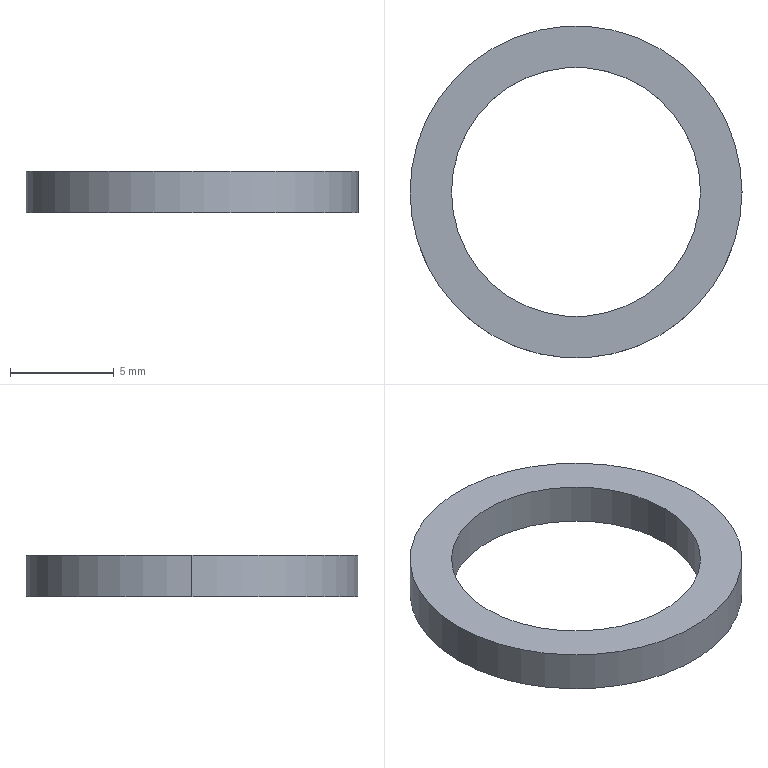Part | SolidWorks | features Extrusion 1 | 1 solid | 6 faces | box 16 x 16 x 2 mm | volume 175.929 mm3 | cylinder 4 | plane 2 | commonest cylinder face diameters 12 x2 16 x2
STEP:
#1=CARTESIAN_POINT('',(-6.,0.,2.));
#2=VERTEX_POINT('',#1);
#3=CARTESIAN_POINT('',(6.,0.,2.));
#4=VERTEX_POINT('',#3);
#5=CARTESIAN_POINT('',(0.,0.,2.));
#6=DIRECTION('',(0.,0.,1.));
#7=DIRECTION('',(1.,0.,0.));
#8=AXIS2_PLACEMENT_3D('',#5,#6,#7);
#9=CIRCLE('',#8,6.);
#10=EDGE_CURVE('',#2,#4,#9,.T.);
#11=ORIENTED_EDGE('',*,*,#10,.T.);
#12=CARTESIAN_POINT('',(6.,0.,0.));
#13=VERTEX_POINT('',#12);
#14=CARTESIAN_POINT('',(6.,0.,2.));
#15=DIRECTION('',(0.,0.,-1.));
#16=VECTOR('',#15,1000.);
#17=LINE('',#14,#16);
#18=EDGE_CURVE('',#4,#13,#17,.T.);
#19=ORIENTED_EDGE('',*,*,#18,.T.);
#20=CARTESIAN_POINT('',(-6.,0.,0.));
#21=VERTEX_POINT('',#20);
#22=CARTESIAN_POINT('',(0.,0.,0.));
#23=DIRECTION('',(0.,0.,1.));
#24=DIRECTION('',(1.,0.,0.));
#25=AXIS2_PLACEMENT_3D('',#22,#23,#24);
#26=CIRCLE('',#25,6.);
#27=EDGE_CURVE('',#21,#13,#26,.T.);
#28=ORIENTED_EDGE('',*,*,#27,.F.);
#29=CARTESIAN_POINT('',(-6.,0.,2.));
#30=DIRECTION('',(0.,0.,-1.));
#31=VECTOR('',#30,1000.);
#32=LINE('',#29,#31);
#33=EDGE_CURVE('',#2,#21,#32,.T.);
#34=ORIENTED_EDGE('',*,*,#33,.F.);
#35=EDGE_LOOP('',(#11,#19,#28,#34));
#36=FACE_OUTER_BOUND('',#35,.T.);
#37=CARTESIAN_POINT('',(0.,0.,2.));
#38=DIRECTION('',(0.,0.,-1.));
#39=DIRECTION('',(-1.,0.,0.));
#40=AXIS2_PLACEMENT_3D('',#37,#38,#39);
#41=CYLINDRICAL_SURFACE('',#40,6.);
#42=ADVANCED_FACE('',(#36),#41,.F.);
#43=CARTESIAN_POINT('',(8.,0.,2.));
#44=VERTEX_POINT('',#43);
#45=CARTESIAN_POINT('',(-8.,0.,2.));
#46=VERTEX_POINT('',#45);
#47=CARTESIAN_POINT('',(0.,0.,2.));
#48=DIRECTION('',(0.,0.,1.));
#49=DIRECTION('',(1.,0.,0.));
#50=AXIS2_PLACEMENT_3D('',#47,#48,#49);
#51=CIRCLE('',#50,8.);
#52=EDGE_CURVE('',#44,#46,#51,.T.);
#53=ORIENTED_EDGE('',*,*,#52,.F.);
#54=CARTESIAN_POINT('',(8.,0.,0.));
#55=VERTEX_POINT('',#54);
#56=CARTESIAN_POINT('',(8.,0.,2.));
#57=DIRECTION('',(0.,0.,-1.));
#58=VECTOR('',#57,1000.);
#59=LINE('',#56,#58);
#60=EDGE_CURVE('',#44,#55,#59,.T.);
#61=ORIENTED_EDGE('',*,*,#60,.T.);
#62=CARTESIAN_POINT('',(-8.,0.,0.));
#63=VERTEX_POINT('',#62);
#64=CARTESIAN_POINT('',(0.,0.,0.));
#65=DIRECTION('',(0.,0.,1.));
#66=DIRECTION('',(1.,0.,0.));
#67=AXIS2_PLACEMENT_3D('',#64,#65,#66);
#68=CIRCLE('',#67,8.);
#69=EDGE_CURVE('',#55,#63,#68,.T.);
#70=ORIENTED_EDGE('',*,*,#69,.T.);
#71=CARTESIAN_POINT('',(-8.,0.,2.));
#72=DIRECTION('',(0.,0.,-1.));
#73=VECTOR('',#72,1000.);
#74=LINE('',#71,#73);
#75=EDGE_CURVE('',#46,#63,#74,.T.);
#76=ORIENTED_EDGE('',*,*,#75,.F.);
#77=EDGE_LOOP('',(#53,#61,#70,#76));
#78=FACE_OUTER_BOUND('',#77,.T.);
#79=CARTESIAN_POINT('',(0.,0.,2.));
#80=DIRECTION('',(0.,0.,-1.));
#81=DIRECTION('',(-1.,0.,0.));
#82=AXIS2_PLACEMENT_3D('',#79,#80,#81);
#83=CYLINDRICAL_SURFACE('',#82,8.);
#84=ADVANCED_FACE('',(#78),#83,.T.);
#85=CARTESIAN_POINT('',(0.,0.,2.));
#86=DIRECTION('',(0.,0.,1.));
#87=DIRECTION('',(1.,0.,0.));
#88=AXIS2_PLACEMENT_3D('',#85,#86,#87);
#89=CIRCLE('',#88,8.);
#90=EDGE_CURVE('',#46,#44,#89,.T.);
#91=ORIENTED_EDGE('',*,*,#90,.T.);
#92=ORIENTED_EDGE('',*,*,#52,.T.);
#93=EDGE_LOOP('',(#91,#92));
#94=FACE_OUTER_BOUND('',#93,.T.);
#95=ORIENTED_EDGE('',*,*,#10,.F.);
#96=CARTESIAN_POINT('',(0.,0.,2.));
#97=DIRECTION('',(0.,0.,1.));
#98=DIRECTION('',(1.,0.,0.));
#99=AXIS2_PLACEMENT_3D('',#96,#97,#98);
#100=CIRCLE('',#99,6.);
#101=EDGE_CURVE('',#4,#2,#100,.T.);
#102=ORIENTED_EDGE('',*,*,#101,.F.);
#103=EDGE_LOOP('',(#95,#102));
#104=FACE_BOUND('',#103,.T.);
#105=CARTESIAN_POINT('',(0.,0.,2.));
#106=DIRECTION('',(0.,0.,1.));
#107=DIRECTION('',(1.,0.,0.));
#108=AXIS2_PLACEMENT_3D('',#105,#106,#107);
#109=PLANE('',#108);
#110=ADVANCED_FACE('',(#94,#104),#109,.T.);
#111=CARTESIAN_POINT('',(0.,0.,0.));
#112=DIRECTION('',(0.,0.,1.));
#113=DIRECTION('',(1.,0.,0.));
#114=AXIS2_PLACEMENT_3D('',#111,#112,#113);
#115=CIRCLE('',#114,8.);
#116=EDGE_CURVE('',#63,#55,#115,.T.);
#117=ORIENTED_EDGE('',*,*,#116,.F.);
#118=ORIENTED_EDGE('',*,*,#69,.F.);
#119=EDGE_LOOP('',(#117,#118));
#120=FACE_OUTER_BOUND('',#119,.T.);
#121=ORIENTED_EDGE('',*,*,#27,.T.);
#122=CARTESIAN_POINT('',(0.,0.,0.));
#123=DIRECTION('',(0.,0.,1.));
#124=DIRECTION('',(1.,0.,0.));
#125=AXIS2_PLACEMENT_3D('',#122,#123,#124);
#126=CIRCLE('',#125,6.);
#127=EDGE_CURVE('',#13,#21,#126,.T.);
#128=ORIENTED_EDGE('',*,*,#127,.T.);
#129=EDGE_LOOP('',(#121,#128));
#130=FACE_BOUND('',#129,.T.);
#131=CARTESIAN_POINT('',(0.,0.,0.));
#132=DIRECTION('',(0.,0.,1.));
#133=DIRECTION('',(1.,0.,0.));
#134=AXIS2_PLACEMENT_3D('',#131,#132,#133);
#135=PLANE('',#134);
#136=ADVANCED_FACE('',(#120,#130),#135,.F.);
#137=ORIENTED_EDGE('',*,*,#60,.F.);
#138=ORIENTED_EDGE('',*,*,#90,.F.);
#139=ORIENTED_EDGE('',*,*,#75,.T.);
#140=ORIENTED_EDGE('',*,*,#116,.T.);
#141=EDGE_LOOP('',(#137,#138,#139,#140));
#142=FACE_OUTER_BOUND('',#141,.T.);
#143=CARTESIAN_POINT('',(0.,0.,2.));
#144=DIRECTION('',(0.,0.,-1.));
#145=DIRECTION('',(-1.,0.,0.));
#146=AXIS2_PLACEMENT_3D('',#143,#144,#145);
#147=CYLINDRICAL_SURFACE('',#146,8.);
#148=ADVANCED_FACE('',(#142),#147,.T.);
#149=ORIENTED_EDGE('',*,*,#18,.F.);
#150=ORIENTED_EDGE('',*,*,#101,.T.);
#151=ORIENTED_EDGE('',*,*,#33,.T.);
#152=ORIENTED_EDGE('',*,*,#127,.F.);
#153=EDGE_LOOP('',(#149,#150,#151,#152));
#154=FACE_OUTER_BOUND('',#153,.T.);
#155=CARTESIAN_POINT('',(0.,0.,2.));
#156=DIRECTION('',(0.,0.,-1.));
#157=DIRECTION('',(-1.,0.,0.));
#158=AXIS2_PLACEMENT_3D('',#155,#156,#157);
#159=CYLINDRICAL_SURFACE('',#158,6.);
#160=ADVANCED_FACE('',(#154),#159,.F.);
#161=CLOSED_SHELL('',(#42,#84,#110,#136,#148,#160));
#162=MANIFOLD_SOLID_BREP('',#161);
#163=CARTESIAN_POINT('',(0.,0.,0.));
#164=DIRECTION('',(0.,0.,1.));
#165=DIRECTION('',(1.,0.,0.));
#166=AXIS2_PLACEMENT_3D('',#163,#164,#165);
#167=(LENGTH_UNIT()NAMED_UNIT(*)SI_UNIT(.MILLI.,.METRE.));
#168=UNCERTAINTY_MEASURE_WITH_UNIT(LENGTH_MEASURE(0.00001),#167,'','');
#169=(NAMED_UNIT(*)PLANE_ANGLE_UNIT()SI_UNIT($,.RADIAN.));
#170=(NAMED_UNIT(*)SI_UNIT($,.STERADIAN.)SOLID_ANGLE_UNIT());
#171=(GEOMETRIC_REPRESENTATION_CONTEXT(3)GLOBAL_UNCERTAINTY_ASSIGNED_CONTEXT((#168))GLOBAL_UNIT_ASSIGNED_CONTEXT((#167,#169,#170))REPRESENTATION_CONTEXT('',''));
#172=ADVANCED_BREP_SHAPE_REPRESENTATION('',(#162,#166),#171);